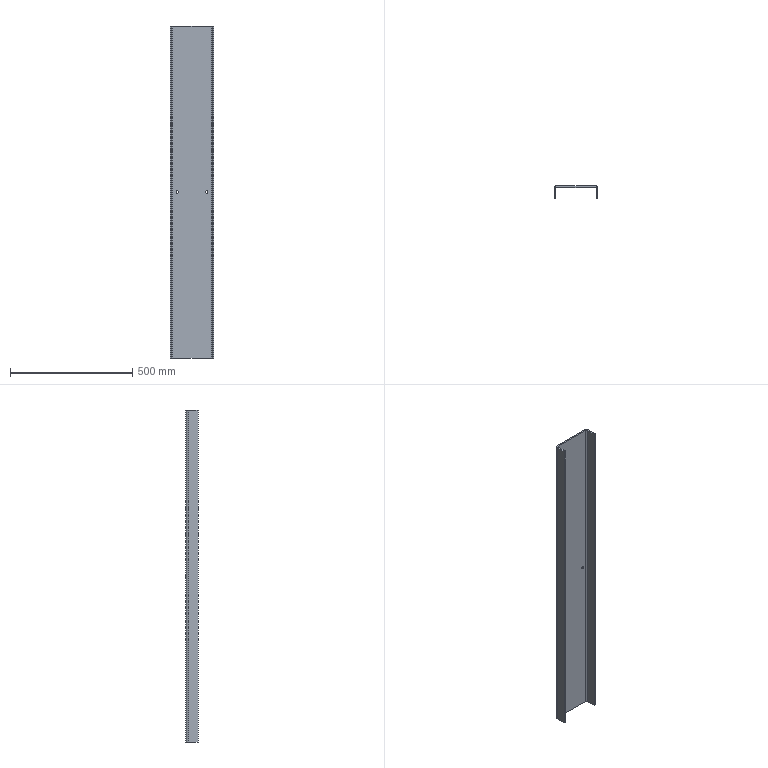Part | STEP file | VD-SYL0380DJ1006_1_1_4-1_VD-SYL | 1 solid | 18 faces | box 180 x 50 x 1360 mm | volume 2129804 mm3 | plane 10 | cylinder 8 | commonest cylinder face diameters 10.5 x4 10 x2 22 x2
STEP:
#1=CARTESIAN_POINT('',(-60.,44.,5.25));
#2=VERTEX_POINT('',#1);
#3=CARTESIAN_POINT('',(-60.,44.,-5.25));
#4=VERTEX_POINT('',#3);
#5=CARTESIAN_POINT('',(-60.,44.,0.));
#6=DIRECTION('',(0.,1.,0.));
#7=DIRECTION('',(0.,0.,1.));
#8=AXIS2_PLACEMENT_3D('',#5,#6,#7);
#9=CIRCLE('',#8,5.25);
#10=EDGE_CURVE('',#2,#4,#9,.T.);
#11=ORIENTED_EDGE('',*,*,#10,.F.);
#12=CARTESIAN_POINT('',(-60.,50.,5.25));
#13=VERTEX_POINT('',#12);
#14=CARTESIAN_POINT('',(-60.,50.,5.25));
#15=DIRECTION('',(0.,-1.,0.));
#16=VECTOR('',#15,1000.);
#17=LINE('',#14,#16);
#18=EDGE_CURVE('',#13,#2,#17,.T.);
#19=ORIENTED_EDGE('',*,*,#18,.F.);
#20=CARTESIAN_POINT('',(-60.,50.,-5.25));
#21=VERTEX_POINT('',#20);
#22=CARTESIAN_POINT('',(-60.,50.,0.));
#23=DIRECTION('',(0.,-1.,0.));
#24=DIRECTION('',(0.,0.,-1.));
#25=AXIS2_PLACEMENT_3D('',#22,#23,#24);
#26=CIRCLE('',#25,5.25);
#27=EDGE_CURVE('',#21,#13,#26,.T.);
#28=ORIENTED_EDGE('',*,*,#27,.F.);
#29=CARTESIAN_POINT('',(-60.,50.,-5.25));
#30=DIRECTION('',(0.,-1.,0.));
#31=VECTOR('',#30,1000.);
#32=LINE('',#29,#31);
#33=EDGE_CURVE('',#21,#4,#32,.T.);
#34=ORIENTED_EDGE('',*,*,#33,.T.);
#35=EDGE_LOOP('',(#11,#19,#28,#34));
#36=FACE_OUTER_BOUND('',#35,.T.);
#37=CARTESIAN_POINT('',(-60.,47.,0.));
#38=DIRECTION('',(0.,1.,0.));
#39=DIRECTION('',(0.,0.,1.));
#40=AXIS2_PLACEMENT_3D('',#37,#38,#39);
#41=CYLINDRICAL_SURFACE('',#40,5.25);
#42=ADVANCED_FACE('',(#36),#41,.F.);
#43=ORIENTED_EDGE('',*,*,#33,.F.);
#44=CARTESIAN_POINT('',(-60.,50.,0.));
#45=DIRECTION('',(0.,-1.,0.));
#46=DIRECTION('',(0.,0.,1.));
#47=AXIS2_PLACEMENT_3D('',#44,#45,#46);
#48=CIRCLE('',#47,5.25);
#49=EDGE_CURVE('',#13,#21,#48,.T.);
#50=ORIENTED_EDGE('',*,*,#49,.F.);
#51=ORIENTED_EDGE('',*,*,#18,.T.);
#52=CARTESIAN_POINT('',(-60.,44.,0.));
#53=DIRECTION('',(0.,1.,0.));
#54=DIRECTION('',(0.,0.,-1.));
#55=AXIS2_PLACEMENT_3D('',#52,#53,#54);
#56=CIRCLE('',#55,5.25);
#57=EDGE_CURVE('',#4,#2,#56,.T.);
#58=ORIENTED_EDGE('',*,*,#57,.F.);
#59=EDGE_LOOP('',(#43,#50,#51,#58));
#60=FACE_OUTER_BOUND('',#59,.T.);
#61=CARTESIAN_POINT('',(-60.,47.,0.));
#62=DIRECTION('',(0.,1.,0.));
#63=DIRECTION('',(0.,0.,1.));
#64=AXIS2_PLACEMENT_3D('',#61,#62,#63);
#65=CYLINDRICAL_SURFACE('',#64,5.25);
#66=ADVANCED_FACE('',(#60),#65,.F.);
#67=CARTESIAN_POINT('',(60.,44.,5.25));
#68=VERTEX_POINT('',#67);
#69=CARTESIAN_POINT('',(60.,44.,-5.25));
#70=VERTEX_POINT('',#69);
#71=CARTESIAN_POINT('',(60.,44.,0.));
#72=DIRECTION('',(0.,1.,0.));
#73=DIRECTION('',(0.,0.,1.));
#74=AXIS2_PLACEMENT_3D('',#71,#72,#73);
#75=CIRCLE('',#74,5.25);
#76=EDGE_CURVE('',#68,#70,#75,.T.);
#77=ORIENTED_EDGE('',*,*,#76,.F.);
#78=CARTESIAN_POINT('',(60.,50.,5.25));
#79=VERTEX_POINT('',#78);
#80=CARTESIAN_POINT('',(60.,50.,5.25));
#81=DIRECTION('',(0.,-1.,0.));
#82=VECTOR('',#81,1000.);
#83=LINE('',#80,#82);
#84=EDGE_CURVE('',#79,#68,#83,.T.);
#85=ORIENTED_EDGE('',*,*,#84,.F.);
#86=CARTESIAN_POINT('',(60.,50.,-5.25));
#87=VERTEX_POINT('',#86);
#88=CARTESIAN_POINT('',(60.,50.,0.));
#89=DIRECTION('',(0.,-1.,0.));
#90=DIRECTION('',(0.,0.,-1.));
#91=AXIS2_PLACEMENT_3D('',#88,#89,#90);
#92=CIRCLE('',#91,5.25);
#93=EDGE_CURVE('',#87,#79,#92,.T.);
#94=ORIENTED_EDGE('',*,*,#93,.F.);
#95=CARTESIAN_POINT('',(60.,50.,-5.25));
#96=DIRECTION('',(0.,-1.,0.));
#97=VECTOR('',#96,1000.);
#98=LINE('',#95,#97);
#99=EDGE_CURVE('',#87,#70,#98,.T.);
#100=ORIENTED_EDGE('',*,*,#99,.T.);
#101=EDGE_LOOP('',(#77,#85,#94,#100));
#102=FACE_OUTER_BOUND('',#101,.T.);
#103=CARTESIAN_POINT('',(60.,47.,0.));
#104=DIRECTION('',(0.,1.,0.));
#105=DIRECTION('',(0.,0.,1.));
#106=AXIS2_PLACEMENT_3D('',#103,#104,#105);
#107=CYLINDRICAL_SURFACE('',#106,5.25);
#108=ADVANCED_FACE('',(#102),#107,.F.);
#109=CARTESIAN_POINT('',(-84.,0.,680.));
#110=VERTEX_POINT('',#109);
#111=CARTESIAN_POINT('',(-84.,0.,-680.));
#112=VERTEX_POINT('',#111);
#113=CARTESIAN_POINT('',(-84.,0.,680.));
#114=DIRECTION('',(0.,0.,-1.));
#115=VECTOR('',#114,1000.);
#116=LINE('',#113,#115);
#117=EDGE_CURVE('',#110,#112,#116,.T.);
#118=ORIENTED_EDGE('',*,*,#117,.T.);
#119=CARTESIAN_POINT('',(-84.,39.,-680.));
#120=VERTEX_POINT('',#119);
#121=CARTESIAN_POINT('',(-84.,0.,-680.));
#122=DIRECTION('',(0.,1.,0.));
#123=VECTOR('',#122,1000.);
#124=LINE('',#121,#123);
#125=EDGE_CURVE('',#112,#120,#124,.T.);
#126=ORIENTED_EDGE('',*,*,#125,.T.);
#127=CARTESIAN_POINT('',(-84.,39.,680.));
#128=VERTEX_POINT('',#127);
#129=CARTESIAN_POINT('',(-84.,39.,680.));
#130=DIRECTION('',(0.,0.,-1.));
#131=VECTOR('',#130,1000.);
#132=LINE('',#129,#131);
#133=EDGE_CURVE('',#128,#120,#132,.T.);
#134=ORIENTED_EDGE('',*,*,#133,.F.);
#135=CARTESIAN_POINT('',(-84.,39.,680.));
#136=DIRECTION('',(0.,-1.,0.));
#137=VECTOR('',#136,1000.);
#138=LINE('',#135,#137);
#139=EDGE_CURVE('',#128,#110,#138,.T.);
#140=ORIENTED_EDGE('',*,*,#139,.T.);
#141=EDGE_LOOP('',(#118,#126,#134,#140));
#142=FACE_OUTER_BOUND('',#141,.T.);
#143=CARTESIAN_POINT('',(-84.,50.,-680.));
#144=DIRECTION('',(-1.,0.,0.));
#145=DIRECTION('',(0.,0.,1.));
#146=AXIS2_PLACEMENT_3D('',#143,#144,#145);
#147=PLANE('',#146);
#148=ADVANCED_FACE('',(#142),#147,.F.);
#149=CARTESIAN_POINT('',(-90.,0.,-680.));
#150=VERTEX_POINT('',#149);
#151=CARTESIAN_POINT('',(-90.,0.,680.));
#152=VERTEX_POINT('',#151);
#153=CARTESIAN_POINT('',(-90.,0.,-680.));
#154=DIRECTION('',(0.,0.,1.));
#155=VECTOR('',#154,1000.);
#156=LINE('',#153,#155);
#157=EDGE_CURVE('',#150,#152,#156,.T.);
#158=ORIENTED_EDGE('',*,*,#157,.F.);
#159=CARTESIAN_POINT('',(-90.,0.,-680.));
#160=DIRECTION('',(1.,0.,0.));
#161=VECTOR('',#160,1000.);
#162=LINE('',#159,#161);
#163=EDGE_CURVE('',#150,#112,#162,.T.);
#164=ORIENTED_EDGE('',*,*,#163,.T.);
#165=ORIENTED_EDGE('',*,*,#117,.F.);
#166=CARTESIAN_POINT('',(-90.,0.,680.));
#167=DIRECTION('',(1.,0.,0.));
#168=VECTOR('',#167,1000.);
#169=LINE('',#166,#168);
#170=EDGE_CURVE('',#152,#110,#169,.T.);
#171=ORIENTED_EDGE('',*,*,#170,.F.);
#172=EDGE_LOOP('',(#158,#164,#165,#171));
#173=FACE_OUTER_BOUND('',#172,.T.);
#174=CARTESIAN_POINT('',(-87.,0.,0.));
#175=DIRECTION('',(0.,-1.,0.));
#176=DIRECTION('',(0.,0.,-1.));
#177=AXIS2_PLACEMENT_3D('',#174,#175,#176);
#178=PLANE('',#177);
#179=ADVANCED_FACE('',(#173),#178,.T.);
#180=CARTESIAN_POINT('',(-90.,39.,-680.));
#181=VERTEX_POINT('',#180);
#182=CARTESIAN_POINT('',(-90.,39.,-680.));
#183=DIRECTION('',(0.,-1.,0.));
#184=VECTOR('',#183,1000.);
#185=LINE('',#182,#184);
#186=EDGE_CURVE('',#181,#150,#185,.T.);
#187=ORIENTED_EDGE('',*,*,#186,.T.);
#188=ORIENTED_EDGE('',*,*,#157,.T.);
#189=CARTESIAN_POINT('',(-90.,39.,680.));
#190=VERTEX_POINT('',#189);
#191=CARTESIAN_POINT('',(-90.,39.,680.));
#192=DIRECTION('',(0.,-1.,0.));
#193=VECTOR('',#192,1000.);
#194=LINE('',#191,#193);
#195=EDGE_CURVE('',#190,#152,#194,.T.);
#196=ORIENTED_EDGE('',*,*,#195,.F.);
#197=CARTESIAN_POINT('',(-90.,39.,-680.));
#198=DIRECTION('',(0.,0.,1.));
#199=VECTOR('',#198,1000.);
#200=LINE('',#197,#199);
#201=EDGE_CURVE('',#181,#190,#200,.T.);
#202=ORIENTED_EDGE('',*,*,#201,.F.);
#203=EDGE_LOOP('',(#187,#188,#196,#202));
#204=FACE_OUTER_BOUND('',#203,.T.);
#205=CARTESIAN_POINT('',(-90.,50.,-680.));
#206=DIRECTION('',(-1.,0.,0.));
#207=DIRECTION('',(0.,0.,1.));
#208=AXIS2_PLACEMENT_3D('',#205,#206,#207);
#209=PLANE('',#208);
#210=ADVANCED_FACE('',(#204),#209,.T.);
#211=ORIENTED_EDGE('',*,*,#201,.T.);
#212=CARTESIAN_POINT('',(-79.,50.,680.));
#213=VERTEX_POINT('',#212);
#214=CARTESIAN_POINT('',(-79.,39.,680.));
#215=DIRECTION('',(0.,0.,1.));
#216=DIRECTION('',(0.,1.,0.));
#217=AXIS2_PLACEMENT_3D('',#214,#215,#216);
#218=CIRCLE('',#217,11.);
#219=EDGE_CURVE('',#213,#190,#218,.T.);
#220=ORIENTED_EDGE('',*,*,#219,.F.);
#221=CARTESIAN_POINT('',(-79.,50.,-680.));
#222=VERTEX_POINT('',#221);
#223=CARTESIAN_POINT('',(-79.,50.,680.));
#224=DIRECTION('',(0.,0.,-1.));
#225=VECTOR('',#224,1000.);
#226=LINE('',#223,#225);
#227=EDGE_CURVE('',#213,#222,#226,.T.);
#228=ORIENTED_EDGE('',*,*,#227,.T.);
#229=CARTESIAN_POINT('',(-79.,39.,-680.));
#230=DIRECTION('',(0.,0.,-1.));
#231=DIRECTION('',(-1.,0.,0.));
#232=AXIS2_PLACEMENT_3D('',#229,#230,#231);
#233=CIRCLE('',#232,11.);
#234=EDGE_CURVE('',#181,#222,#233,.T.);
#235=ORIENTED_EDGE('',*,*,#234,.F.);
#236=EDGE_LOOP('',(#211,#220,#228,#235));
#237=FACE_OUTER_BOUND('',#236,.T.);
#238=CARTESIAN_POINT('',(-79.,39.,-680.));
#239=DIRECTION('',(0.,0.,-1.));
#240=DIRECTION('',(-1.,0.,0.));
#241=AXIS2_PLACEMENT_3D('',#238,#239,#240);
#242=CYLINDRICAL_SURFACE('',#241,11.);
#243=ADVANCED_FACE('',(#237),#242,.T.);
#244=ORIENTED_EDGE('',*,*,#27,.T.);
#245=ORIENTED_EDGE('',*,*,#49,.T.);
#246=EDGE_LOOP('',(#244,#245));
#247=FACE_BOUND('',#246,.T.);
#248=ORIENTED_EDGE('',*,*,#93,.T.);
#249=CARTESIAN_POINT('',(60.,50.,0.));
#250=DIRECTION('',(0.,-1.,0.));
#251=DIRECTION('',(0.,0.,1.));
#252=AXIS2_PLACEMENT_3D('',#249,#250,#251);
#253=CIRCLE('',#252,5.25);
#254=EDGE_CURVE('',#79,#87,#253,.T.);
#255=ORIENTED_EDGE('',*,*,#254,.T.);
#256=EDGE_LOOP('',(#248,#255));
#257=FACE_BOUND('',#256,.T.);
#258=CARTESIAN_POINT('',(79.,50.,-680.));
#259=VERTEX_POINT('',#258);
#260=CARTESIAN_POINT('',(79.,50.,-680.));
#261=DIRECTION('',(-1.,0.,0.));
#262=VECTOR('',#261,1000.);
#263=LINE('',#260,#262);
#264=EDGE_CURVE('',#259,#222,#263,.T.);
#265=ORIENTED_EDGE('',*,*,#264,.T.);
#266=ORIENTED_EDGE('',*,*,#227,.F.);
#267=CARTESIAN_POINT('',(79.,50.,680.));
#268=VERTEX_POINT('',#267);
#269=CARTESIAN_POINT('',(79.,50.,680.));
#270=DIRECTION('',(-1.,0.,0.));
#271=VECTOR('',#270,1000.);
#272=LINE('',#269,#271);
#273=EDGE_CURVE('',#268,#213,#272,.T.);
#274=ORIENTED_EDGE('',*,*,#273,.F.);
#275=CARTESIAN_POINT('',(79.,50.,-680.));
#276=DIRECTION('',(0.,0.,1.));
#277=VECTOR('',#276,1000.);
#278=LINE('',#275,#277);
#279=EDGE_CURVE('',#259,#268,#278,.T.);
#280=ORIENTED_EDGE('',*,*,#279,.F.);
#281=EDGE_LOOP('',(#265,#266,#274,#280));
#282=FACE_OUTER_BOUND('',#281,.T.);
#283=CARTESIAN_POINT('',(90.,50.,-680.));
#284=DIRECTION('',(0.,1.,0.));
#285=DIRECTION('',(1.,0.,0.));
#286=AXIS2_PLACEMENT_3D('',#283,#284,#285);
#287=PLANE('',#286);
#288=ADVANCED_FACE('',(#247,#257,#282),#287,.T.);
#289=ORIENTED_EDGE('',*,*,#279,.T.);
#290=CARTESIAN_POINT('',(90.,39.,680.));
#291=VERTEX_POINT('',#290);
#292=CARTESIAN_POINT('',(79.,39.,680.));
#293=DIRECTION('',(0.,0.,1.));
#294=DIRECTION('',(1.,0.,0.));
#295=AXIS2_PLACEMENT_3D('',#292,#293,#294);
#296=CIRCLE('',#295,11.);
#297=EDGE_CURVE('',#291,#268,#296,.T.);
#298=ORIENTED_EDGE('',*,*,#297,.F.);
#299=CARTESIAN_POINT('',(90.,39.,-680.));
#300=VERTEX_POINT('',#299);
#301=CARTESIAN_POINT('',(90.,39.,680.));
#302=DIRECTION('',(0.,0.,-1.));
#303=VECTOR('',#302,1000.);
#304=LINE('',#301,#303);
#305=EDGE_CURVE('',#291,#300,#304,.T.);
#306=ORIENTED_EDGE('',*,*,#305,.T.);
#307=CARTESIAN_POINT('',(79.,39.,-680.));
#308=DIRECTION('',(0.,0.,-1.));
#309=DIRECTION('',(0.,1.,0.));
#310=AXIS2_PLACEMENT_3D('',#307,#308,#309);
#311=CIRCLE('',#310,11.);
#312=EDGE_CURVE('',#259,#300,#311,.T.);
#313=ORIENTED_EDGE('',*,*,#312,.F.);
#314=EDGE_LOOP('',(#289,#298,#306,#313));
#315=FACE_OUTER_BOUND('',#314,.T.);
#316=CARTESIAN_POINT('',(79.,39.,-680.));
#317=DIRECTION('',(0.,0.,-1.));
#318=DIRECTION('',(-1.,0.,0.));
#319=AXIS2_PLACEMENT_3D('',#316,#317,#318);
#320=CYLINDRICAL_SURFACE('',#319,11.);
#321=ADVANCED_FACE('',(#315),#320,.T.);
#322=CARTESIAN_POINT('',(90.,0.,-680.));
#323=VERTEX_POINT('',#322);
#324=CARTESIAN_POINT('',(90.,0.,-680.));
#325=DIRECTION('',(0.,1.,0.));
#326=VECTOR('',#325,1000.);
#327=LINE('',#324,#326);
#328=EDGE_CURVE('',#323,#300,#327,.T.);
#329=ORIENTED_EDGE('',*,*,#328,.T.);
#330=ORIENTED_EDGE('',*,*,#305,.F.);
#331=CARTESIAN_POINT('',(90.,0.,680.));
#332=VERTEX_POINT('',#331);
#333=CARTESIAN_POINT('',(90.,0.,680.));
#334=DIRECTION('',(0.,1.,0.));
#335=VECTOR('',#334,1000.);
#336=LINE('',#333,#335);
#337=EDGE_CURVE('',#332,#291,#336,.T.);
#338=ORIENTED_EDGE('',*,*,#337,.F.);
#339=CARTESIAN_POINT('',(90.,0.,-680.));
#340=DIRECTION('',(0.,0.,1.));
#341=VECTOR('',#340,1000.);
#342=LINE('',#339,#341);
#343=EDGE_CURVE('',#323,#332,#342,.T.);
#344=ORIENTED_EDGE('',*,*,#343,.F.);
#345=EDGE_LOOP('',(#329,#330,#338,#344));
#346=FACE_OUTER_BOUND('',#345,.T.);
#347=CARTESIAN_POINT('',(90.,0.,-680.));
#348=DIRECTION('',(1.,0.,0.));
#349=DIRECTION('',(0.,1.,0.));
#350=AXIS2_PLACEMENT_3D('',#347,#348,#349);
#351=PLANE('',#350);
#352=ADVANCED_FACE('',(#346),#351,.T.);
#353=CARTESIAN_POINT('',(84.,0.,-680.));
#354=VERTEX_POINT('',#353);
#355=CARTESIAN_POINT('',(84.,0.,-680.));
#356=DIRECTION('',(1.,0.,0.));
#357=VECTOR('',#356,1000.);
#358=LINE('',#355,#357);
#359=EDGE_CURVE('',#354,#323,#358,.T.);
#360=ORIENTED_EDGE('',*,*,#359,.T.);
#361=ORIENTED_EDGE('',*,*,#343,.T.);
#362=CARTESIAN_POINT('',(84.,0.,680.));
#363=VERTEX_POINT('',#362);
#364=CARTESIAN_POINT('',(90.,0.,680.));
#365=DIRECTION('',(-1.,0.,0.));
#366=VECTOR('',#365,1000.);
#367=LINE('',#364,#366);
#368=EDGE_CURVE('',#332,#363,#367,.T.);
#369=ORIENTED_EDGE('',*,*,#368,.T.);
#370=CARTESIAN_POINT('',(84.,0.,-680.));
#371=DIRECTION('',(0.,0.,1.));
#372=VECTOR('',#371,1000.);
#373=LINE('',#370,#372);
#374=EDGE_CURVE('',#354,#363,#373,.T.);
#375=ORIENTED_EDGE('',*,*,#374,.F.);
#376=EDGE_LOOP('',(#360,#361,#369,#375));
#377=FACE_OUTER_BOUND('',#376,.T.);
#378=CARTESIAN_POINT('',(87.,0.,0.));
#379=DIRECTION('',(0.,1.,0.));
#380=DIRECTION('',(1.,0.,0.));
#381=AXIS2_PLACEMENT_3D('',#378,#379,#380);
#382=PLANE('',#381);
#383=ADVANCED_FACE('',(#377),#382,.F.);
#384=CARTESIAN_POINT('',(84.,39.,-680.));
#385=VERTEX_POINT('',#384);
#386=CARTESIAN_POINT('',(84.,39.,680.));
#387=VERTEX_POINT('',#386);
#388=CARTESIAN_POINT('',(84.,39.,-680.));
#389=DIRECTION('',(0.,0.,1.));
#390=VECTOR('',#389,1000.);
#391=LINE('',#388,#390);
#392=EDGE_CURVE('',#385,#387,#391,.T.);
#393=ORIENTED_EDGE('',*,*,#392,.F.);
#394=CARTESIAN_POINT('',(84.,39.,-680.));
#395=DIRECTION('',(0.,-1.,0.));
#396=VECTOR('',#395,1000.);
#397=LINE('',#394,#396);
#398=EDGE_CURVE('',#385,#354,#397,.T.);
#399=ORIENTED_EDGE('',*,*,#398,.T.);
#400=ORIENTED_EDGE('',*,*,#374,.T.);
#401=CARTESIAN_POINT('',(84.,0.,680.));
#402=DIRECTION('',(0.,1.,0.));
#403=VECTOR('',#402,1000.);
#404=LINE('',#401,#403);
#405=EDGE_CURVE('',#363,#387,#404,.T.);
#406=ORIENTED_EDGE('',*,*,#405,.T.);
#407=EDGE_LOOP('',(#393,#399,#400,#406));
#408=FACE_OUTER_BOUND('',#407,.T.);
#409=CARTESIAN_POINT('',(84.,0.,-680.));
#410=DIRECTION('',(1.,0.,0.));
#411=DIRECTION('',(0.,1.,0.));
#412=AXIS2_PLACEMENT_3D('',#409,#410,#411);
#413=PLANE('',#412);
#414=ADVANCED_FACE('',(#408),#413,.F.);
#415=CARTESIAN_POINT('',(79.,44.,680.));
#416=VERTEX_POINT('',#415);
#417=CARTESIAN_POINT('',(79.,39.,680.));
#418=DIRECTION('',(0.,0.,-1.));
#419=DIRECTION('',(0.,1.,0.));
#420=AXIS2_PLACEMENT_3D('',#417,#418,#419);
#421=CIRCLE('',#420,5.);
#422=EDGE_CURVE('',#416,#387,#421,.T.);
#423=ORIENTED_EDGE('',*,*,#422,.F.);
#424=CARTESIAN_POINT('',(79.,44.,-680.));
#425=VERTEX_POINT('',#424);
#426=CARTESIAN_POINT('',(79.,44.,680.));
#427=DIRECTION('',(0.,0.,-1.));
#428=VECTOR('',#427,1000.);
#429=LINE('',#426,#428);
#430=EDGE_CURVE('',#416,#425,#429,.T.);
#431=ORIENTED_EDGE('',*,*,#430,.T.);
#432=CARTESIAN_POINT('',(79.,39.,-680.));
#433=DIRECTION('',(0.,0.,1.));
#434=DIRECTION('',(1.,0.,0.));
#435=AXIS2_PLACEMENT_3D('',#432,#433,#434);
#436=CIRCLE('',#435,5.);
#437=EDGE_CURVE('',#385,#425,#436,.T.);
#438=ORIENTED_EDGE('',*,*,#437,.F.);
#439=ORIENTED_EDGE('',*,*,#392,.T.);
#440=EDGE_LOOP('',(#423,#431,#438,#439));
#441=FACE_OUTER_BOUND('',#440,.T.);
#442=CARTESIAN_POINT('',(79.,39.,-680.));
#443=DIRECTION('',(0.,0.,-1.));
#444=DIRECTION('',(-1.,0.,0.));
#445=AXIS2_PLACEMENT_3D('',#442,#443,#444);
#446=CYLINDRICAL_SURFACE('',#445,5.);
#447=ADVANCED_FACE('',(#441),#446,.F.);
#448=CARTESIAN_POINT('',(-79.,44.,-680.));
#449=VERTEX_POINT('',#448);
#450=CARTESIAN_POINT('',(-79.,39.,-680.));
#451=DIRECTION('',(0.,0.,1.));
#452=DIRECTION('',(0.,1.,0.));
#453=AXIS2_PLACEMENT_3D('',#450,#451,#452);
#454=CIRCLE('',#453,5.);
#455=EDGE_CURVE('',#449,#120,#454,.T.);
#456=ORIENTED_EDGE('',*,*,#455,.T.);
#457=ORIENTED_EDGE('',*,*,#125,.F.);
#458=ORIENTED_EDGE('',*,*,#163,.F.);
#459=ORIENTED_EDGE('',*,*,#186,.F.);
#460=ORIENTED_EDGE('',*,*,#234,.T.);
#461=ORIENTED_EDGE('',*,*,#264,.F.);
#462=ORIENTED_EDGE('',*,*,#312,.T.);
#463=ORIENTED_EDGE('',*,*,#328,.F.);
#464=ORIENTED_EDGE('',*,*,#359,.F.);
#465=ORIENTED_EDGE('',*,*,#398,.F.);
#466=ORIENTED_EDGE('',*,*,#437,.T.);
#467=CARTESIAN_POINT('',(-79.,44.,-680.));
#468=DIRECTION('',(1.,0.,0.));
#469=VECTOR('',#468,1000.);
#470=LINE('',#467,#469);
#471=EDGE_CURVE('',#449,#425,#470,.T.);
#472=ORIENTED_EDGE('',*,*,#471,.F.);
#473=EDGE_LOOP('',(#456,#457,#458,#459,#460,#461,#462,#463,#464,#465,#466,#472));
#474=FACE_OUTER_BOUND('',#473,.T.);
#475=CARTESIAN_POINT('',(0.,47.,-680.));
#476=DIRECTION('',(0.,0.,-1.));
#477=DIRECTION('',(0.,-1.,0.));
#478=AXIS2_PLACEMENT_3D('',#475,#476,#477);
#479=PLANE('',#478);
#480=ADVANCED_FACE('',(#474),#479,.T.);
#481=CARTESIAN_POINT('',(-79.,44.,680.));
#482=VERTEX_POINT('',#481);
#483=CARTESIAN_POINT('',(-79.,39.,680.));
#484=DIRECTION('',(0.,0.,-1.));
#485=DIRECTION('',(-1.,0.,0.));
#486=AXIS2_PLACEMENT_3D('',#483,#484,#485);
#487=CIRCLE('',#486,5.);
#488=EDGE_CURVE('',#128,#482,#487,.T.);
#489=ORIENTED_EDGE('',*,*,#488,.F.);
#490=ORIENTED_EDGE('',*,*,#133,.T.);
#491=ORIENTED_EDGE('',*,*,#455,.F.);
#492=CARTESIAN_POINT('',(-79.,44.,-680.));
#493=DIRECTION('',(0.,0.,1.));
#494=VECTOR('',#493,1000.);
#495=LINE('',#492,#494);
#496=EDGE_CURVE('',#449,#482,#495,.T.);
#497=ORIENTED_EDGE('',*,*,#496,.T.);
#498=EDGE_LOOP('',(#489,#490,#491,#497));
#499=FACE_OUTER_BOUND('',#498,.T.);
#500=CARTESIAN_POINT('',(-79.,39.,-680.));
#501=DIRECTION('',(0.,0.,-1.));
#502=DIRECTION('',(-1.,0.,0.));
#503=AXIS2_PLACEMENT_3D('',#500,#501,#502);
#504=CYLINDRICAL_SURFACE('',#503,5.);
#505=ADVANCED_FACE('',(#499),#504,.F.);
#506=ORIENTED_EDGE('',*,*,#422,.T.);
#507=ORIENTED_EDGE('',*,*,#405,.F.);
#508=ORIENTED_EDGE('',*,*,#368,.F.);
#509=ORIENTED_EDGE('',*,*,#337,.T.);
#510=ORIENTED_EDGE('',*,*,#297,.T.);
#511=ORIENTED_EDGE('',*,*,#273,.T.);
#512=ORIENTED_EDGE('',*,*,#219,.T.);
#513=ORIENTED_EDGE('',*,*,#195,.T.);
#514=ORIENTED_EDGE('',*,*,#170,.T.);
#515=ORIENTED_EDGE('',*,*,#139,.F.);
#516=ORIENTED_EDGE('',*,*,#488,.T.);
#517=CARTESIAN_POINT('',(79.,44.,680.));
#518=DIRECTION('',(-1.,0.,0.));
#519=VECTOR('',#518,1000.);
#520=LINE('',#517,#519);
#521=EDGE_CURVE('',#416,#482,#520,.T.);
#522=ORIENTED_EDGE('',*,*,#521,.F.);
#523=EDGE_LOOP('',(#506,#507,#508,#509,#510,#511,#512,#513,#514,#515,#516,#522));
#524=FACE_OUTER_BOUND('',#523,.T.);
#525=CARTESIAN_POINT('',(0.,47.,680.));
#526=DIRECTION('',(0.,0.,-1.));
#527=DIRECTION('',(0.,-1.,0.));
#528=AXIS2_PLACEMENT_3D('',#525,#526,#527);
#529=PLANE('',#528);
#530=ADVANCED_FACE('',(#524),#529,.F.);
#531=ORIENTED_EDGE('',*,*,#76,.T.);
#532=CARTESIAN_POINT('',(60.,44.,0.));
#533=DIRECTION('',(0.,1.,0.));
#534=DIRECTION('',(0.,0.,-1.));
#535=AXIS2_PLACEMENT_3D('',#532,#533,#534);
#536=CIRCLE('',#535,5.25);
#537=EDGE_CURVE('',#70,#68,#536,.T.);
#538=ORIENTED_EDGE('',*,*,#537,.T.);
#539=EDGE_LOOP('',(#531,#538));
#540=FACE_BOUND('',#539,.T.);
#541=ORIENTED_EDGE('',*,*,#10,.T.);
#542=ORIENTED_EDGE('',*,*,#57,.T.);
#543=EDGE_LOOP('',(#541,#542));
#544=FACE_BOUND('',#543,.T.);
#545=ORIENTED_EDGE('',*,*,#496,.F.);
#546=ORIENTED_EDGE('',*,*,#471,.T.);
#547=ORIENTED_EDGE('',*,*,#430,.F.);
#548=ORIENTED_EDGE('',*,*,#521,.T.);
#549=EDGE_LOOP('',(#545,#546,#547,#548));
#550=FACE_OUTER_BOUND('',#549,.T.);
#551=CARTESIAN_POINT('',(90.,44.,-680.));
#552=DIRECTION('',(0.,1.,0.));
#553=DIRECTION('',(1.,0.,0.));
#554=AXIS2_PLACEMENT_3D('',#551,#552,#553);
#555=PLANE('',#554);
#556=ADVANCED_FACE('',(#540,#544,#550),#555,.F.);
#557=ORIENTED_EDGE('',*,*,#99,.F.);
#558=ORIENTED_EDGE('',*,*,#254,.F.);
#559=ORIENTED_EDGE('',*,*,#84,.T.);
#560=ORIENTED_EDGE('',*,*,#537,.F.);
#561=EDGE_LOOP('',(#557,#558,#559,#560));
#562=FACE_OUTER_BOUND('',#561,.T.);
#563=CARTESIAN_POINT('',(60.,47.,0.));
#564=DIRECTION('',(0.,1.,0.));
#565=DIRECTION('',(0.,0.,1.));
#566=AXIS2_PLACEMENT_3D('',#563,#564,#565);
#567=CYLINDRICAL_SURFACE('',#566,5.25);
#568=ADVANCED_FACE('',(#562),#567,.F.);
#569=CLOSED_SHELL('',(#42,#66,#108,#148,#179,#210,#243,#288,#321,#352,#383,#414,#447,#480,#505,#530,#556,#568));
#570=MANIFOLD_SOLID_BREP('',#569);
#571=CARTESIAN_POINT('',(0.,0.,0.));
#572=DIRECTION('',(0.,0.,1.));
#573=DIRECTION('',(1.,0.,0.));
#574=AXIS2_PLACEMENT_3D('',#571,#572,#573);
#575=(LENGTH_UNIT()NAMED_UNIT(*)SI_UNIT(.MILLI.,.METRE.));
#576=UNCERTAINTY_MEASURE_WITH_UNIT(LENGTH_MEASURE(0.00001),#575,'','');
#577=(NAMED_UNIT(*)PLANE_ANGLE_UNIT()SI_UNIT($,.RADIAN.));
#578=(NAMED_UNIT(*)SI_UNIT($,.STERADIAN.)SOLID_ANGLE_UNIT());
#579=(GEOMETRIC_REPRESENTATION_CONTEXT(3)GLOBAL_UNCERTAINTY_ASSIGNED_CONTEXT((#576))GLOBAL_UNIT_ASSIGNED_CONTEXT((#575,#577,#578))REPRESENTATION_CONTEXT('',''));
#580=ADVANCED_BREP_SHAPE_REPRESENTATION('',(#570,#574),#579);